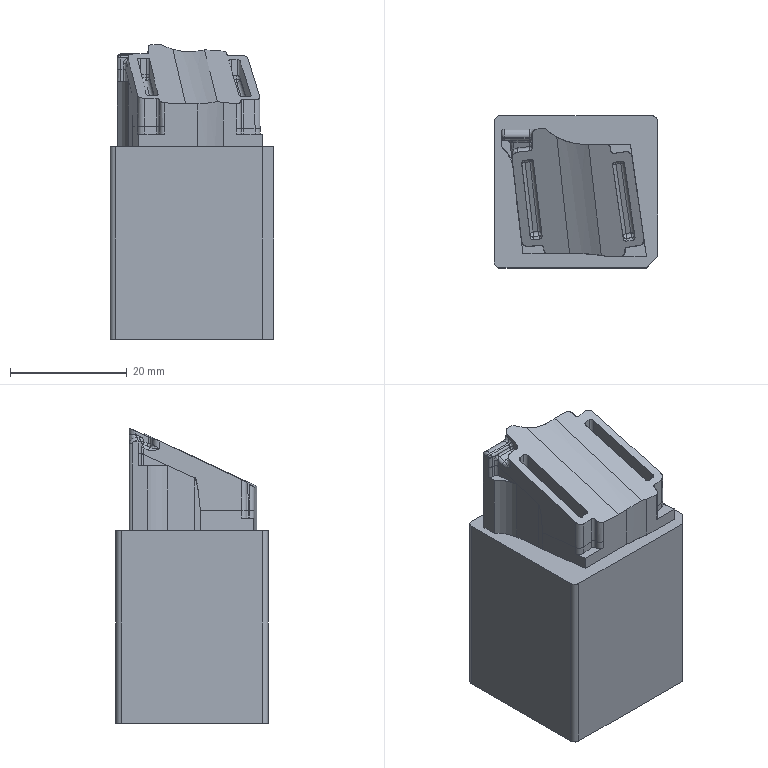NC program | NX | posted with a generic post | part box 28 x 26 x 50.455 mm
Whole program:
N10 G17 G21 G94 G90
(CONTOUR_AREA_1 , TOOL : D0.8R0.4)
N12 T00 M6
N14 G54
N16 G17 G0 G90 X-13.442 Y10.172 S0 M3
N18 G43 Z10. H0
N20 Z1.2
N22 G94 G1 Z-3.351 F250.
N24 X-13.296 Y10.317 Z-3.332
N26 X-13.177 Y10.437 Z-3.212
N28 X-13.116 Y10.498 Z-3.024
N30 X-13.077 Y10.536 Z-2.705
N32 X-13.039 Y10.575 Z-2.609
N34 X-12.962 Y10.652 Z-2.512
N36 X-12.931 Y10.683 Z-2.49
N38 X-12.761 Y10.853 Z-2.513
N40 X-12.628 Y10.986 Z-2.654
N42 X-12.591 Y11.022 Z-2.731
N44 X-12.553 Y11.061 Z-3.024
N46 X-12.381 Y11.093
N48 X-12.456 Y11.018 Z-2.583
N50 X-12.522 Y10.952 Z-2.469
N52 X-12.691 Y10.783 Z-2.308
N54 X-12.861 Y10.613 Z-2.274
N56 X-13.031 Y10.443 Z-2.381
N58 X-13.078 Y10.396 Z-2.465
N60 X-13.15 Y10.324 Z-3.024
N62 X-13.162 Y10.249
N64 X-13.163 Y10.171 Z-2.858
N66 X-13.13 Y10.204 Z-2.474
N68 X-13.102 Y10.232 Z-2.38
N70 X-12.961 Y10.373 Z-2.19
N72 X-12.791 Y10.543 Z-2.121
N74 X-12.621 Y10.713 Z-2.15
N76 X-12.452 Y10.882 Z-2.293
N78 X-12.368 Y10.966 Z-2.418
N80 X-12.282 Y11.052 Z-2.614
N82 X-12.249 Y11.085 Z-2.731
N84 X-12.217 Y11.118 Z-3.024
N86 X-12.077
N88 X-12.107 Y11.088 Z-2.745
N90 X-12.137 Y11.058 Z-2.627
N92 X-12.212 Y10.982 Z-2.437
N94 X-12.382 Y10.813 Z-2.179
N96 X-12.551 Y10.643 Z-2.046
N98 X-12.721 Y10.473 Z-2.005
N100 X-12.891 Y10.303 Z-2.04
N102 X-13.061 Y10.134 Z-2.215
N104 X-13.104 Y10.09 Z-2.295
N106 X-13.164 Y10.03 Z-2.61
N108 Y9.952 Z-2.586
N110 Y9.89 Z-2.531
N112 X-13.104 Y9.95 Z-2.236
N114 X-12.991 Y10.064 Z-2.055
N116 X-12.821 Y10.234 Z-1.943
N118 X-12.651 Y10.403 Z-1.907
N120 X-12.482 Y10.573 Z-1.961
N122 X-12.312 Y10.743 Z-2.075
N124 X-12.142 Y10.912 Z-2.3
N126 X-11.997 Y11.058 Z-2.627
N128 X-11.972 Y11.082 Z-2.716
N130 X-11.937 Y11.118 Z-3.024
N132 X-11.797
N134 X-11.827 Y11.088 Z-2.745
N136 X-11.857 Y11.058 Z-2.627
N138 X-11.903 Y11.012 Z-2.512
N140 X-12.072 Y10.842 Z-2.204
N142 X-12.242 Y10.673 Z-2.008
N144 X-12.412 Y10.503 Z-1.884
N146 X-12.581 Y10.333 Z-1.839
N148 X-12.751 Y10.164 Z-1.853
N150 X-12.921 Y9.994 Z-1.948
N152 X-13.09 Y9.824 Z-2.177
N154 X-13.104 Y9.811 Z-2.209
N156 X-13.164 Y9.751 Z-2.503
N158 Y9.611 Z-2.515
N160 X-13.104 Y9.671 Z-2.207
N162 X-13.021 Y9.754 Z-2.038
N164 X-12.851 Y9.924 Z-1.869
N166 X-12.681 Y10.094 Z-1.786
N168 X-12.511 Y10.263 Z-1.783
N170 X-12.342 Y10.433 Z-1.829
N172 X-12.172 Y10.603 Z-1.95
N174 X-12.002 Y10.773 Z-2.108
N176 X-11.833 Y10.942 Z-2.346
N178 X-11.717 Y11.058 Z-2.627
N180 X-11.687 Y11.088 Z-2.745
N182 X-11.657 Y11.118 Z-3.024
N184 X-11.518
N186 X-11.548 Y11.088 Z-2.745
N188 X-11.578 Y11.058 Z-2.627
N190 X-11.593 Y11.042 Z-2.588
N192 X-11.678 Y10.957 Z-2.375
N194 X-11.763 Y10.872 Z-2.245
N196 X-11.932 Y10.703 Z-2.032
N198 X-12.102 Y10.533 Z-1.892
N200 X-12.272 Y10.363 Z-1.79
N202 X-12.442 Y10.194 Z-1.729
N204 X-12.611 Y10.024 Z-1.736
N206 X-12.781 Y9.854 Z-1.798
N208 X-12.951 Y9.684 Z-1.952
N210 X-13.104 Y9.531 Z-2.225
N212 X-13.12 Y9.515 Z-2.284
N214 X-13.142 Y9.493 Z-2.369
N216 X-13.154 Y9.482 Z-2.439
N218 X-13.165 Y9.471 Z-2.572
N220 Y9.356 Z-2.641
N222 X-13.164 Y9.332 Z-2.62
N224 X-13.105 Y9.391 Z-2.272
N226 X-13.051 Y9.445 Z-2.137
N228 X-12.881 Y9.615 Z-1.88
N230 X-12.711 Y9.784 Z-1.747
N232 X-12.541 Y9.954 Z-1.699
N234 X-12.372 Y10.124 Z-1.694
N236 X-12.202 Y10.293 Z-1.757
N238 X-12.032 Y10.463 Z-1.839
N240 X-11.863 Y10.633 Z-1.975
N242 X-11.693 Y10.803 Z-2.149
N244 X-11.523 Y10.972 Z-2.411
N246 X-11.438 Y11.058 Z-2.627
N248 X-11.408 Y11.088 Z-2.745
N250 X-11.378 Y11.118 Z-3.024
N252 X-11.238
N254 X-11.261 Y11.095 Z-2.783
N256 X-11.284 Y11.072 Z-2.67
N258 X-11.298 Y11.058 Z-2.627
N260 X-11.453 Y10.902 Z-2.286
N262 X-11.623 Y10.733 Z-2.06
N264 X-11.793 Y10.563 Z-1.917
N266 X-11.962 Y10.393 Z-1.804
N268 X-12.132 Y10.223 Z-1.724
N270 X-12.302 Y10.054 Z-1.673
N272 X-12.471 Y9.884 Z-1.664
N274 X-12.641 Y9.714 Z-1.71
N276 X-12.811 Y9.545 Z-1.827
N278 X-12.981 Y9.375 Z-2.046
N280 X-13.04 Y9.315 Z-2.16
N282 X-13.1 Y9.256 Z-2.319
N284 X-13.157 Y9.198 Z-2.68
N286 X-13.152 Y9.092 Z-2.706
N288 X-13.15 Y9.066 Z-2.687
N290 X-13.094 Y9.122 Z-2.364
N292 X-13.08 Y9.135 Z-2.327
N294 X-13.002 Y9.214 Z-2.156
N296 X-12.996 Y9.22 Z-2.139
N298 X-12.911 Y9.305 Z-1.981
N300 X-12.741 Y9.475 Z-1.785
N302 X-12.571 Y9.644 Z-1.681
N304 X-12.402 Y9.814 Z-1.639
N306 X-12.232 Y9.984 Z-1.658
N308 X-12.062 Y10.154 Z-1.694
N310 X-11.892 Y10.323 Z-1.771
N312 X-11.723 Y10.493 Z-1.86
N314 X-11.553 Y10.663 Z-1.999
N316 X-11.383 Y10.832 Z-2.19
N318 X-11.214 Y11.002 Z-2.487
N320 X-11.158 Y11.058 Z-2.627
N322 X-11.128 Y11.088 Z-2.745
N324 X-11.098 Y11.118 Z-3.024
N326 X-10.958
N328 X-10.988 Y11.088 Z-2.745
N330 X-11.018 Y11.058 Z-2.627
N332 X-11.144 Y10.932 Z-2.329
N334 X-11.313 Y10.763 Z-2.094
N336 X-11.483 Y10.593 Z-1.941
N338 X-11.653 Y10.423 Z-1.818
N340 X-11.823 Y10.253 Z-1.738
N342 X-11.992 Y10.084 Z-1.677
N344 X-12.162 Y9.914 Z-1.644
N346 X-12.332 Y9.744 Z-1.631
N348 X-12.501 Y9.575 Z-1.669
N350 X-12.671 Y9.405 Z-1.766
N352 X-12.841 Y9.235 Z-1.939
N354 X-12.926 Y9.15 Z-2.065
N356 X-12.991 Y9.085 Z-2.199
N358 X-13.011 Y9.065 Z-2.232
N360 X-13.066 Y9.01 Z-2.367
N362 X-13.112 Y8.964 Z-2.705
N364 X-13.073 Y8.863
N366 X-13.027 Y8.91 Z-2.344
N368 X-12.941 Y8.996 Z-2.158
N370 X-12.843 Y9.093 Z-2.009
N372 X-12.8 Y9.136 Z-1.957
N374 X-12.771 Y9.165 Z-1.91
N376 X-12.601 Y9.335 Z-1.753
N378 X-12.432 Y9.505 Z-1.658
N380 X-12.262 Y9.674 Z-1.626
N382 X-12.092 Y9.844 Z-1.631
N384 X-11.922 Y10.014 Z-1.664
N386 X-11.753 Y10.184 Z-1.705
N388 X-11.583 Y10.353 Z-1.785
N390 X-11.413 Y10.523 Z-1.884
N392 X-11.244 Y10.693 Z-2.024
N394 X-11.074 Y10.862 Z-2.231
N396 X-10.904 Y11.032 Z-2.562
N398 X-10.879 Y11.058 Z-2.627
N400 X-10.849 Y11.088 Z-2.745
N402 X-10.819 Y11.118 Z-3.024
N404 X-10.679
N406 X-10.709 Y11.088 Z-2.745
N408 X-10.739 Y11.058 Z-2.627
N410 X-10.834 Y10.962 Z-2.386
N412 X-11.004 Y10.792 Z-2.135
N414 X-11.174 Y10.623 Z-1.966
N416 X-11.343 Y10.453 Z-1.833
N418 X-11.513 Y10.283 Z-1.752
N420 X-11.683 Y10.114 Z-1.683
N422 X-11.853 Y9.944 Z-1.65
N424 X-12.022 Y9.774 Z-1.626
N426 X-12.192 Y9.605 Z-1.629
N428 X-12.362 Y9.435 Z-1.661
N430 X-12.531 Y9.265 Z-1.752
N432 X-12.701 Y9.095 Z-1.903
N434 X-12.871 Y8.926 Z-2.11
N436 X-12.987 Y8.809 Z-2.375
N438 X-13.011 Y8.786 Z-2.464
N440 X-13.034 Y8.763 Z-2.665
N442 X-13.033 Y8.761 Z-2.704
N444 X-12.976 Y8.681 Z-2.668
N446 X-12.955 Y8.702 Z-2.478
N448 X-12.933 Y8.724 Z-2.375
N450 X-12.801 Y8.856 Z-2.085
N452 X-12.631 Y9.025 Z-1.889
N454 X-12.461 Y9.195 Z-1.753
N456 X-12.292 Y9.365 Z-1.676
N458 X-12.122 Y9.535 Z-1.638
N460 X-11.952 Y9.704 Z-1.626
N462 X-11.783 Y9.874 Z-1.637
N464 X-11.613 Y10.044 Z-1.669
N466 X-11.443 Y10.213 Z-1.719
N468 X-11.273 Y10.383 Z-1.799
N470 X-11.104 Y10.553 Z-1.908
N472 X-10.934 Y10.723 Z-2.05
N474 X-10.764 Y10.892 Z-2.273
N476 X-10.595 Y11.062 Z-2.638
N478 X-10.567 Y11.09 Z-2.757
N480 X-10.539 Y11.118 Z-3.024
N482 X-10.399
N484 X-10.429 Y11.088 Z-2.745
N486 X-10.459 Y11.058 Z-2.627
N488 X-10.525 Y10.992 Z-2.461
N490 X-10.694 Y10.822 Z-2.176
N492 X-10.864 Y10.653 Z-1.991
N494 X-11.034 Y10.483 Z-1.852
N496 X-11.204 Y10.313 Z-1.766
N498 X-11.373 Y10.144 Z-1.691
N500 X-11.543 Y9.974 Z-1.656
N502 X-11.713 Y9.804 Z-1.627
N504 X-11.882 Y9.634
N506 X-12.052 Y9.465 Z-1.647
N508 X-12.222 Y9.295 Z-1.698
N510 X-12.392 Y9.125 Z-1.767
N512 X-12.561 Y8.956 Z-1.893
N514 X-12.731 Y8.786 Z-2.073
N516 X-12.868 Y8.648 Z-2.376
N518 X-12.911 Y8.606 Z-2.703
N520 X-12.862 Y8.553
N522 X-12.84 Y8.537 Z-2.659
N524 X-12.819 Y8.558 Z-2.477
N526 X-12.797 Y8.58 Z-2.387
N528 X-12.661 Y8.716 Z-2.081
N530 X-12.491 Y8.886 Z-1.909
N532 X-12.322 Y9.055 Z-1.793
N534 X-12.152 Y9.225 Z-1.72
N536 X-11.982 Y9.395 Z-1.665
N538 X-11.813 Y9.565 Z-1.634
N540 X-11.643 Y9.734 Z-1.626
N542 X-11.473 Y9.904 Z-1.642
N544 X-11.303 Y10.074 Z-1.675
N546 X-11.134 Y10.243 Z-1.733
N548 X-10.964 Y10.413 Z-1.813
N550 X-10.794 Y10.583 Z-1.933
N552 X-10.625 Y10.752 Z-2.082
N554 X-10.455 Y10.922 Z-2.314
N556 X-10.319 Y11.058 Z-2.627
N558 X-10.285 Y11.092 Z-2.767
N560 X-10.259 Y11.118 Z-3.024
N562 X-10.12
N564 X-10.15 Y11.088 Z-2.745
N566 X-10.18 Y11.058 Z-2.627
N568 X-10.215 Y11.022 Z-2.537
N570 X-10.385 Y10.852 Z-2.218
N572 X-10.555 Y10.683 Z-2.016
N574 X-10.724 Y10.513 Z-1.875
N576 X-10.894 Y10.343 Z-1.78
N578 X-11.064 Y10.173 Z-1.701
N580 X-11.234 Y10.004 Z-1.662
N582 X-11.403 Y9.834 Z-1.63
N584 X-11.573 Y9.664 Z-1.626
N586 X-11.743 Y9.495 Z-1.643
N588 X-11.912 Y9.325 Z-1.688
N590 X-12.082 Y9.155 Z-1.743
N592 X-12.124 Y9.113 Z-1.762
N594 X-12.262 Y8.975 Z-1.826
N596 X-12.379 Y8.858 Z-1.897
N598 X-12.421 Y8.816 Z-1.929
N600 X-12.591 Y8.646 Z-2.099
N602 X-12.717 Y8.521 Z-2.391
N604 X-12.738 Y8.499 Z-2.468
N606 X-12.76 Y8.478 Z-2.67
N608 X-12.74 Y8.463 Z-2.703
N610 X-12.669 Y8.429
N612 X-12.624 Y8.474 Z-2.378
N614 X-12.521 Y8.576 Z-2.143
N616 X-12.352 Y8.746 Z-1.953
N618 X-12.245 Y8.852 Z-1.884
N620 X-11.98 Y9.117 Z-1.76
N622 X-11.842 Y9.255 Z-1.711
N624 X-11.673 Y9.425 Z-1.656
N626 X-11.503 Y9.594 Z-1.631
N628 X-11.333 Y9.764 Z-1.626
N630 X-11.164 Y9.934 Z-1.648
N632 X-10.994 Y10.104 Z-1.681
N634 X-10.824 Y10.273 Z-1.747
N636 X-10.655 Y10.443 Z-1.828
N638 X-10.485 Y10.613 Z-1.958
N640 X-10.315 Y10.782 Z-2.121
N642 X-10.145 Y10.952 Z-2.364
N644 X-10.04 Y11.058 Z-2.627
N646 X-10.01 Y11.088 Z-2.745
N648 X-9.98 Y11.118 Z-3.024
N650 X-9.84
N652 X-9.87 Y11.088 Z-2.745
N654 X-9.906 Y11.052 Z-2.613
N656 X-9.991 Y10.967 Z-2.398
N658 X-10.075 Y10.882 Z-2.259
N660 X-10.245 Y10.712 Z-2.041
N662 X-10.415 Y10.543 Z-1.9
N664 X-10.585 Y10.373 Z-1.794
N666 X-10.754 Y10.203 Z-1.714
N668 X-10.924 Y10.034 Z-1.667
N670 X-11.094 Y9.864 Z-1.635
N672 X-11.263 Y9.694 Z-1.626
N674 X-11.433 Y9.525 Z-1.639
N676 X-11.603 Y9.355 Z-1.678
N678 X-11.773 Y9.185 Z-1.733
N680 X-11.836 Y9.121 Z-1.757
N682 X-12.101 Y8.856 Z-1.882
N684 X-12.112 Y8.846 Z-1.887
N686 X-12.196 Y8.761 Z-1.94
N688 X-12.282 Y8.676 Z-1.992
N690 X-12.451 Y8.506 Z-2.2
N692 X-12.528 Y8.43 Z-2.393
N694 X-12.574 Y8.383 Z-2.659
N696 X-12.555 Y8.374 Z-2.703
N698 X-12.461 Y8.357 Z-2.907
N700 X-12.409 Y8.409 Z-2.369
N702 X-12.381 Y8.436 Z-2.301
N704 X-12.212 Y8.606 Z-2.054
N706 X-12.042 Y8.776 Z-1.929
N708 X-11.968 Y8.85 Z-1.885
N710 X-11.703 Y9.115 Z-1.76
N712 X-11.533 Y9.285 Z-1.701
N714 X-11.363 Y9.455 Z-1.649
N716 X-11.194 Y9.624 Z-1.627
N718 X-11.024 Y9.794 Z-1.626
N720 X-10.854 Y9.964 Z-1.654
N722 X-10.684 Y10.133 Z-1.688
N724 X-10.515 Y10.303 Z-1.761
N726 X-10.345 Y10.473 Z-1.845
N728 X-10.175 Y10.643 Z-1.983
N730 X-10.006 Y10.812 Z-2.162
N732 X-9.836 Y10.982 Z-2.436
N734 X-9.76 Y11.058 Z-2.627
N736 X-9.73 Y11.088 Z-2.745
N738 X-9.7 Y11.118 Z-3.024
N740 X-9.56
N742 X-9.596 Y11.082 Z-2.715
N744 X-9.62 Y11.058 Z-2.627
N746 X-9.766 Y10.912 Z-2.3
N748 X-9.936 Y10.742 Z-2.07
N750 X-10.105 Y10.573 Z-1.925
N752 X-10.275 Y10.403 Z-1.808
N754 X-10.445 Y10.233 Z-1.728
N756 X-10.615 Y10.064 Z-1.673
N758 X-10.784 Y9.894 Z-1.641
N760 X-10.954 Y9.724 Z-1.626
N762 X-11.124 Y9.554 Z-1.636
N764 X-11.293 Y9.385 Z-1.669
N766 X-11.463 Y9.215 Z-1.724
N768 X-11.548 Y9.13 Z-1.753
N770 X-11.559 Y9.12 Z-1.758
N772 X-11.824 Y8.854 Z-1.883
N774 X-11.887 Y8.791 Z-1.918
N776 X-11.972 Y8.706 Z-1.98
N778 X-12.142 Y8.536 Z-2.129
N780 X-12.291 Y8.387 Z-2.381
N782 X-12.312 Y8.367 Z-2.447
N784 X-12.342 Y8.336 Z-3.163
N786 X-12.274 Y8.323 Z-3.311
N788 X-12.247 Y8.322 Z-3.667
N790 X-12.216 Z-3.744
N792 X-12.202 Y8.337 Z-2.571
N794 X-12.187 Y8.352 Z-2.499
N796 X-12.157 Y8.381 Z-2.395
N798 X-12.072 Y8.466 Z-2.222
N800 X-11.902 Y8.636 Z-2.03
N802 X-11.733 Y8.806 Z-1.908
N804 X-11.69 Y8.848 Z-1.886
N806 X-11.425 Y9.113 Z-1.761
N808 X-11.414 Y9.124 Z-1.756
N810 X-11.393 Y9.145 Z-1.747
N812 X-11.223 Y9.315 Z-1.691
N814 X-11.054 Y9.485 Z-1.644
N816 X-10.884 Y9.654 Z-1.626
N818 X-10.714 Y9.824 Z-1.629
N820 X-10.545 Y9.994 Z-1.66
N822 X-10.375 Y10.163 Z-1.697
N824 X-10.205 Y10.333 Z-1.775
N826 X-10.036 Y10.503 Z-1.867
N828 X-9.866 Y10.673 Z-2.007
N830 X-9.696 Y10.842 Z-2.204
N832 X-9.526 Y11.012 Z-2.512
N834 X-9.481 Y11.058 Z-2.627
N836 X-9.451 Y11.088 Z-2.745
N838 X-9.421 Y11.118 Z-3.024
N840 X-9.281
N842 X-9.311 Y11.088 Z-2.745
N844 X-9.341 Y11.058 Z-2.627
N846 X-9.456 Y10.942 Z-2.345
N848 X-9.626 Y10.772 Z-2.107
N850 X-9.796 Y10.603 Z-1.95
N852 X-9.966 Y10.433 Z-1.822
N854 X-10.135 Y10.263 Z-1.742
N856 X-10.305 Y10.093 Z-1.679
N858 X-10.475 Y9.924 Z-1.646
N860 X-10.644 Y9.754 Z-1.626
N862 X-10.814 Y9.584 Z-1.632
N864 X-10.984 Y9.415 Z-1.659
N866 X-11.154 Y9.245 Z-1.714
N868 X-11.281 Y9.118 Z-1.759
N870 X-11.546 Y8.853 Z-1.884
N872 X-11.557 Y8.842 Z-1.889
N874 X-11.578 Y8.821 Z-1.9
N876 X-11.663 Y8.736 Z-1.958
N878 X-11.832 Y8.566 Z-2.092
N880 X-12.002 Y8.396 Z-2.357
N882 X-12.018 Y8.38 Z-2.399
N884 X-12.048 Y8.35 Z-2.507
N886 X-12.063 Y8.336 Z-2.582
N888 X-12.078 Y8.321 Z-4.086
N890 X-11.939 Y8.319 Z-4.631
N892 X-11.924 Y8.334 Z-2.592
N894 X-11.909 Y8.349 Z-2.515
N896 X-11.879 Y8.379 Z-2.402
N898 X-11.762 Y8.496 Z-2.181
N900 X-11.593 Y8.666 Z-2.008
N902 X-11.423 Y8.836 Z-1.892
N904 X-11.412 Y8.846 Z-1.887
N906 X-11.402 Y8.857 Z-1.882
N908 X-11.137 Y9.122 Z-1.757
N910 X-11.126 Y9.133 Z-1.752
N912 X-11.084 Y9.175 Z-1.737
N914 X-10.914 Y9.345 Z-1.682
N916 X-10.744 Y9.514 Z-1.641
N918 X-10.575 Y9.684 Z-1.626
N920 X-10.405 Y9.854 Z-1.633
N922 X-10.235 Y10.024 Z-1.665
N924 X-10.065 Y10.193 Z-1.709
N926 X-9.896 Y10.363 Z-1.789
N928 X-9.726 Y10.533 Z-1.892
N930 X-9.556 Y10.702 Z-2.032
N932 X-9.387 Y10.872 Z-2.245
N934 X-9.302 Y10.957 Z-2.375
N936 X-9.217 Y11.042 Z-2.587
N938 X-9.201 Y11.058 Z-2.627
N940 X-9.171 Y11.088 Z-2.745
N942 X-9.141 Y11.118 Z-3.024
N944 X-9.001
N946 X-9.031 Y11.088 Z-2.745
N948 X-9.061 Y11.058 Z-2.627
N950 X-9.147 Y10.972 Z-2.411
N952 X-9.317 Y10.802 Z-2.149
N954 X-9.486 Y10.633 Z-1.974
N956 X-9.656 Y10.463 Z-1.839
N958 X-9.826 Y10.293 Z-1.756
N960 X-9.996 Y10.123 Z-1.685
N962 X-10.165 Y9.954 Z-1.652
N964 X-10.335 Y9.784 Z-1.626
N966 X-10.505 Y9.614 Z-1.628
N968 X-10.674 Y9.445 Z-1.651
N970 X-10.844 Y9.275 Z-1.704
N972 X-11.003 Y9.116 Z-1.76
N974 X-11.268 Y8.851 Z-1.885
N976 X-11.353 Y8.766 Z-1.935
N978 X-11.523 Y8.596 Z-2.062
N980 X-11.693 Y8.426 Z-2.297
N982 X-11.741 Y8.378 Z-2.404
N984 X-11.785 Y8.334 Z-2.597
N986 X-11.8 Y8.319 Z-3.985
N988 X-11.747
N990 X-11.686 Y8.294 Z-3.7
N992 Y8.293 Z-3.702
N994 X-11.656 Y8.323 Z-3.195
N996 X-11.653 Y8.326 Z-2.68
N998 X-11.643 Y8.336 Z-2.582
N1000 X-11.623 Y8.356 Z-2.499
N1002 X-11.538 Y8.441 Z-2.267
N1004 X-11.453 Y8.526 Z-2.142
N1006 X-11.283 Y8.696 Z-1.986
N1008 X-11.198 Y8.781 Z-1.924
N1010 X-11.156 Y8.823 Z-1.898
N1012 X-11.135 Y8.844 Z-1.888
N1014 X-11.124 Y8.855 Z-1.883
N1016 X-10.859 Y9.12 Z-1.758
N1018 X-10.774 Y9.205 Z-1.727
N1020 X-10.604 Y9.375 Z-1.672
N1022 X-10.435 Y9.544 Z-1.637
N1024 X-10.265 Y9.714 Z-1.626
N1026 X-10.095 Y9.884 Z-1.639
N1028 X-9.926 Y10.054 Z-1.671
N1030 X-9.756 Y10.223 Z-1.724
N1032 X-9.586 Y10.393 Z-1.803
N1034 X-9.417 Y10.563 Z-1.916
N1036 X-9.247 Y10.732 Z-2.06
N1038 X-9.077 Y10.902 Z-2.286
N1040 X-8.922 Y11.058 Z-2.627
N1042 X-8.907 Y11.072 Z-2.669
N1044 X-8.884 Y11.095 Z-2.782
N1046 X-8.862 Y11.118 Z-3.024
N1048 X-8.722
N1050 X-8.752 Y11.088 Z-2.745
N1052 X-8.782 Y11.058 Z-2.627
N1054 X-8.838 Y11.002 Z-2.486
N1056 X-9.007 Y10.832 Z-2.19
N1058 X-9.177 Y10.662 Z-1.999
N1060 X-9.347 Y10.493 Z-1.859
N1062 X-9.516 Y10.323 Z-1.771
N1064 X-9.686 Y10.153 Z-1.694
N1066 X-9.856 Y9.984 Z-1.658
N1068 X-10.025 Y9.814 Z-1.628
N1070 X-10.195 Y9.644 Z-1.626
N1072 X-10.365 Y9.474 Z-1.646
N1074 X-10.535 Y9.305 Z-1.695
N1076 X-10.704 Y9.135 Z-1.751
N1078 X-10.715 Y9.124 Z-1.756
N1080 X-10.725 Y9.114 Z-1.761
N1082 X-10.991 Y8.849 Z-1.886
N1084 X-11.001 Y8.838 Z-1.891
N1086 X-11.044 Y8.796 Z-1.914
N1088 X-11.213 Y8.626 Z-2.037
N1090 X-11.383 Y8.456 Z-2.239
N1092 X-11.468 Y8.371 Z-2.428
N1094 X-11.51 Y8.329 Z-2.651
N1096 X-11.521 Y8.318 Z-3.042
N1098 X-11.532 Y8.308 Z-3.117
N1100 X-11.553 Y8.287 Z-3.237
N1102 X-11.594 Y8.245 Z-3.372
N1104 X-11.62 Y8.219 Z-3.489
N1106 X-11.646 Y8.193 Z-3.724
N1108 X-11.632 Y8.068 Z-3.787
N1110 X-11.577 Y8.122 Z-3.422
N1112 X-11.483 Y8.217 Z-3.169
N1114 X-11.429 Y8.271 Z-3.051
N1116 X-11.402 Y8.298 Z-2.993
N1118 X-11.375 Y8.325 Z-2.844
N1120 X-11.359 Y8.34 Z-2.564
N1122 X-11.344 Y8.356 Z-2.503
N1124 X-11.313 Y8.386 Z-2.382
N1126 X-11.143 Y8.556 Z-2.105
N1128 X-10.974 Y8.726 Z-1.964
N1130 X-10.857 Y8.842 Z-1.889
N1132 X-10.847 Y8.853 Z-1.884
N1134 X-10.581 Y9.118 Z-1.759
N1136 X-10.465 Y9.235 Z-1.717
N1138 X-10.295 Y9.405 Z-1.662
N1140 X-10.125 Y9.574 Z-1.633
N1142 X-9.956 Y9.744 Z-1.626
N1144 X-9.786 Y9.914 Z-1.644
N1146 X-9.616 Y10.083 Z-1.677
N1148 X-9.446 Y10.253 Z-1.738
N1150 X-9.277 Y10.423 Z-1.818
N1152 X-9.107 Y10.593 Z-1.941
N1154 X-8.937 Y10.762 Z-2.094
N1156 X-8.768 Y10.932 Z-2.329
N1158 X-8.642 Y11.058 Z-2.627
N1160 X-8.612 Y11.088 Z-2.745
N1162 X-8.582 Y11.118 Z-3.024
N1164 X-8.442
N1166 X-8.472 Y11.088 Z-2.745
N1168 X-8.502 Y11.058 Z-2.627
N1170 X-8.528 Y11.032 Z-2.562
N1172 X-8.698 Y10.862 Z-2.231
N1174 X-8.867 Y10.692 Z-2.024
N1176 X-9.037 Y10.523 Z-1.883
N1178 X-9.207 Y10.353 Z-1.785
N1180 X-9.377 Y10.183 Z-1.705
N1182 X-9.546 Y10.014 Z-1.663
N1184 X-9.716 Y9.844 Z-1.631
N1186 X-9.886 Y9.674 Z-1.626
N1188 X-10.055 Y9.504 Z-1.642
N1190 X-10.225 Y9.335 Z-1.685
N1192 X-10.395 Y9.165 Z-1.74
N1194 X-10.437 Y9.123 Z-1.757
N1196 X-10.448 Y9.112 Z-1.762
N1198 X-10.702 Y8.857 Z-1.881
N1200 X-10.713 Y8.847 Z-1.886
N1202 X-10.734 Y8.826 Z-1.897
N1204 X-10.904 Y8.656 Z-2.015
N1206 X-11.074 Y8.486 Z-2.194
N1208 X-11.158 Y8.401 Z-2.348
N1210 X-11.201 Y8.359 Z-2.486
N1212 X-11.222 Y8.338 Z-2.579
N1214 X-11.234 Y8.326 Z-2.705
N1216 X-11.243 Y8.316 Z-2.826
N1218 X-11.286 Y8.274 Z-2.917
N1220 X-11.328 Y8.232 Z-2.983
N1222 X-11.413 Y8.147 Z-3.12
N1224 X-11.563 Y7.997 Z-3.48
N1226 X-11.583 Y7.977 Z-3.572
N1228 X-11.617 Y7.943 Z-3.832
N1230 X-11.602 Y7.818 Z-3.886
N1232 X-11.548 Y7.872 Z-3.536
N1234 X-11.513 Y7.907 Z-3.433
N1236 X-11.343 Y8.077 Z-3.085
N1238 X-11.173 Y8.247 Z-2.866
N1240 X-11.131 Y8.289 Z-2.816
N1242 X-11.11 Y8.31 Z-2.783
N1244 X-11.105 Y8.315 Z-2.77
N1246 X-11.099 Y8.321 Z-2.75
N1248 Z-2.748
N1250 X-11.094 Y8.326 Z-2.699
N1252 X-11.089 Y8.331 Z-2.617
N1254 X-11.004 Y8.416 Z-2.316
N1256 X-10.834 Y8.586 Z-2.072
N1258 X-10.664 Y8.756 Z-1.941
N1260 X-10.579 Y8.841 Z-1.889
N1262 X-10.569 Y8.851 Z-1.884
N1264 X-10.304 Y9.116 Z-1.76
N1266 X-10.155 Y9.265 Z-1.708
N1268 X-9.985 Y9.435 Z-1.654
N1270 X-9.816 Y9.604 Z-1.629
N1272 X-9.646 Y9.774 Z-1.626
N1274 X-9.476 Y9.944 Z-1.65
N1276 X-9.307 Y10.113 Z-1.683
N1278 X-9.137 Y10.283 Z-1.752
N1280 X-8.967 Y10.453 Z-1.833
N1282 X-8.798 Y10.622 Z-1.966
N1284 X-8.628 Y10.792 Z-2.135
N1286 X-8.458 Y10.962 Z-2.386
N1288 X-8.362 Y11.058 Z-2.627
N1290 X-8.332 Y11.088 Z-2.745
N1292 X-8.302 Y11.118 Z-3.024
N1294 X-8.163
N1296 X-8.191 Y11.09 Z-2.756
N1298 X-8.219 Y11.062 Z-2.638
N1300 X-8.388 Y10.892 Z-2.272
N1302 X-8.558 Y10.722 Z-2.05
N1304 X-8.728 Y10.553 Z-1.908
N1306 X-8.897 Y10.383 Z-1.799
N1308 X-9.067 Y10.213 Z-1.719
N1310 X-9.237 Y10.043 Z-1.669
N1312 X-9.406 Y9.874 Z-1.637
N1314 X-9.576 Y9.704 Z-1.626
N1316 X-9.746 Y9.534 Z-1.638
N1318 X-9.916 Y9.365 Z-1.675
N1320 X-10.085 Y9.195 Z-1.73
N1322 X-10.16 Y9.121 Z-1.758
N1324 X-10.425 Y8.856 Z-1.882
N1326 X-10.51 Y8.771 Z-1.93
N1328 X-10.594 Y8.686 Z-1.993
N1330 X-10.764 Y8.516 Z-2.155
N1332 X-10.849 Y8.431 Z-2.287
N1334 X-10.934 Y8.346 Z-2.546
N1336 X-10.955 Y8.325 Z-2.668
N1338 X-10.977 Y8.304 Z-2.746
N1340 X-10.998 Y8.282 Z-2.773
N1342 X-11.041 Y8.239 Z-2.815
N1344 X-11.104 Y8.177 Z-2.869
N1346 X-11.273 Y8.007 Z-3.064
N1348 X-11.443 Y7.837 Z-3.348
N1350 X-11.534 Y7.747 Z-3.594
N1352 X-11.588 Y7.692 Z-3.945
N1354 X-11.573 Y7.567 Z-4.004
N1356 X-11.543 Y7.598 Z-3.763
N1358 X-11.519 Y7.621 Z-3.651
N1360 X-11.373 Y7.767 Z-3.299
N1362 X-11.203 Y7.937 Z-3.05
N1364 X-11.034 Y8.107 Z-2.879
N1366 X-10.949 Y8.192 Z-2.815
N1368 X-10.864 Y8.276 Z-2.754
N1370 X-10.821 Y8.319 Z-2.691
N1372 X-10.779 Y8.361 Z-2.471
N1374 X-10.694 Y8.446 Z-2.258
N1376 X-10.524 Y8.616 Z-2.044
N1378 X-10.355 Y8.786 Z-1.92
N1380 X-10.291 Y8.849 Z-1.885
N1382 X-10.026 Y9.114 Z-1.761
N1384 X-10.015 Y9.125 Z-1.756
N1386 X-9.846 Y9.295 Z-1.698
N1388 X-9.676 Y9.464 Z-1.647
N1390 X-9.506 Y9.634 Z-1.627
N1392 X-9.337 Y9.804
N1394 X-9.167 Y9.974 Z-1.656
N1396 X-8.997 Y10.143 Z-1.691
N1398 X-8.827 Y10.313 Z-1.766
N1400 X-8.658 Y10.483 Z-1.852
N1402 X-8.488 Y10.652 Z-1.991
N1404 X-8.318 Y10.822 Z-2.176
N1406 X-8.149 Y10.992 Z-2.461
N1408 X-8.083 Y11.058 Z-2.627
N1410 X-8.053 Y11.088 Z-2.745
N1412 X-8.023 Y11.118 Z-3.024
N1414 X-7.883 Z-3.007
N1416 X-7.909 Y11.092 Z-2.75
N1418 X-7.943 Y11.058 Z-2.637
N1420 X-8.011 Y10.99 Z-2.445
N1422 X-8.028 Y10.973 Z-2.405
N1424 X-8.079 Y10.922 Z-2.313
N1426 X-8.248 Y10.752 Z-2.082
N1428 X-8.418 Y10.582 Z-1.933
N1430 X-8.588 Y10.413 Z-1.813
N1432 X-8.758 Y10.243 Z-1.733
N1434 X-8.927 Y10.073 Z-1.675
N1436 X-9.097 Y9.904 Z-1.642
N1438 X-9.267 Y9.734 Z-1.626
N1440 X-9.436 Y9.564 Z-1.634
N1442 X-9.606 Y9.395 Z-1.666
N1444 X-9.776 Y9.225 Z-1.721
N1446 X-9.882 Y9.119 Z-1.759
N1448 X-10.147 Y8.854 Z-1.883
N1450 X-10.158 Y8.843 Z-1.888
N1452 X-10.2 Y8.801 Z-1.911
N1454 X-10.285 Y8.716 Z-1.971
N1456 X-10.455 Y8.546 Z-2.118
N1458 X-10.624 Y8.376 Z-2.41
N1460 X-10.675 Y8.326 Z-2.649
N1462 X-10.704 Y8.296 Z-2.731
N1464 X-10.764 Y8.236 Z-2.774
N1466 X-10.779 Y8.222 Z-2.781
N1468 X-10.794 Y8.207 Z-2.788
N1470 X-10.964 Y8.037 Z-2.891
N1472 X-11.133 Y7.867 Z-3.044
N1474 X-11.303 Y7.697 Z-3.263
N1476 X-11.473 Y7.528 Z-3.614
N1478 X-11.505 Y7.496 Z-3.709
N1480 X-11.559 Y7.442 Z-4.059
N1482 X-11.544 Y7.317 Z-4.109
N1484 X-11.53 Y7.33 Z-3.956
N1486 X-11.49 Y7.371 Z-3.766
N1488 X-11.403 Y7.458 Z-3.528
N1490 X-11.233 Y7.628 Z-3.24
N1492 X-11.064 Y7.797 Z-3.045
N1494 X-10.894 Y7.967 Z-2.913
N1496 X-10.756 Y8.105 Z-2.834
N1498 X-10.629 Y8.232 Z-2.776
N1500 X-10.618 Y8.243 Z-2.77
N1502 X-10.597 Y8.264 Z-2.757
N1504 X-10.554 Y8.306 Z-2.719
N1506 X-10.512 Y8.349 Z-2.531
N1508 X-10.47 Y8.391 Z-2.372
N1510 X-10.385 Y8.476 Z-2.208
N1512 X-10.215 Y8.646 Z-2.021
N1514 X-10.045 Y8.816 Z-1.902
N1516 X-10.003 Y8.858 Z-1.881
N1518 X-9.748 Y9.113 Z-1.762
N1520 X-9.706 Y9.155 Z-1.743
N1522 X-9.536 Y9.325 Z-1.688
N1524 X-9.366 Y9.494 Z-1.643
N1526 X-9.197 Y9.664 Z-1.626
N1528 X-9.027 Y9.834 Z-1.63
N1530 X-8.857 Y10.003 Z-1.662
N1532 X-8.688 Y10.173 Z-1.701
N1534 X-8.518 Y10.343 Z-1.78
N1536 X-8.348 Y10.513 Z-1.875
N1538 X-8.179 Y10.682 Z-2.016
N1540 X-8.009 Y10.852 Z-2.217
N1542 X-7.988 Y10.873 Z-2.247
N1544 X-7.924 Y10.937 Z-2.327
N1546 X-7.839 Y11.022 Z-2.513
N1548 X-7.803 Y11.058 Z-2.603
N1550 X-7.773 Y11.088 Z-2.717
N1552 X-7.743 Y11.118 Z-2.994
N1554 X-7.636 Z-2.968
N1556 X-7.603 Z-2.955
N1558 X-7.633 Y11.088 Z-2.67
N1560 X-7.663 Y11.058 Z-2.557
N1562 X-7.769 Y10.952 Z-2.315
N1564 X-7.939 Y10.782 Z-2.113
N1566 X-8.109 Y10.612 Z-1.958
N1568 X-8.278 Y10.443 Z-1.828
N1570 X-8.448 Y10.273 Z-1.747
N1572 X-8.618 Y10.103 Z-1.681
N1574 X-8.787 Y9.934 Z-1.648
N1576 X-8.957 Y9.764 Z-1.626
N1578 X-9.127 Y9.594 Z-1.631
N1580 X-9.297 Y9.424 Z-1.656
N1582 X-9.466 Y9.255 Z-1.711
N1584 X-9.604 Y9.117 Z-1.76
N1586 X-9.869 Y8.852 Z-1.884
N1588 X-9.975 Y8.746 Z-1.948
N1590 X-10.145 Y8.576 Z-2.082
N1592 X-10.315 Y8.406 Z-2.339
N1594 X-10.395 Y8.326 Z-2.649
N1596 X-10.417 Y8.304 Z-2.723
N1598 X-10.44 Y8.281 Z-2.746
N1600 X-10.485 Y8.237 Z-2.774
N1602 X-10.75 Y7.971 Z-2.895
N1604 X-10.824 Y7.897 Z-2.936
N1606 X-10.994 Y7.727 Z-3.055
N1608 X-11.163 Y7.558 Z-3.225
N1610 X-11.333 Y7.388 Z-3.478
N1612 X-11.404 Y7.317 Z-3.621
N1614 X-11.475 Y7.246 Z-3.817
N1616 X-11.503 Y7.218 Z-3.923
N1618 X-11.529 Y7.192 Z-4.149
N1620 X-11.515 Y7.067 Z-4.176
N1622 X-11.46 Y7.121 Z-3.848
N1624 X-11.433 Y7.148 Z-3.771
N1626 X-11.263 Y7.318 Z-3.441
N1628 X-11.093 Y7.488 Z-3.221
N1630 X-10.924 Y7.657 Z-3.066
N1632 X-10.754 Y7.827 Z-2.962
N1634 X-10.743 Y7.838 Z-2.956
N1636 X-10.733 Y7.848 Z-2.951
N1638 X-10.355 Y8.226 Z-2.778
N1640 X-10.335 Y8.246 Z-2.768
N1642 X-10.295 Y8.286 Z-2.742
N1644 X-10.255 Y8.326 Z-2.649
N1646 X-10.245 Y8.336 Z-2.592
N1648 X-10.16 Y8.421 Z-2.306
N1650 X-10.075 Y8.506 Z-2.169
N1652 X-9.905 Y8.676 Z-1.999
N1654 X-9.736 Y8.845 Z-1.887
N1656 X-9.725 Y8.856 Z-1.882
N1658 X-9.46 Y9.121 Z-1.758
N1660 X-9.396 Y9.185 Z-1.733
N1662 X-9.227 Y9.355 Z-1.678
N1664 X-9.057 Y9.524 Z-1.639
N1666 X-8.887 Y9.694 Z-1.626
N1668 X-8.718 Y9.864 Z-1.635
N1670 X-8.548 Y10.033 Z-1.667
N1672 X-8.378 Y10.203 Z-1.714
N1674 X-8.208 Y10.373 Z-1.794
N1676 X-8.039 Y10.542 Z-1.9
N1678 X-7.996 Y10.585 Z-1.93
N1680 X-7.954 Y10.627 Z-1.96
N1682 X-7.869 Y10.712 Z-2.01
N1684 X-7.699 Y10.882 Z-2.167
N1686 X-7.53 Y11.052 Z-2.478
N1688 X-7.494 Y11.088 Z-2.61
N1690 X-7.464 Y11.118 Z-2.905
N1692 X-7.324 Z-2.836
N1694 X-7.354 Y11.088 Z-2.522
N1696 X-7.384 Y11.058 Z-2.406
N1698 X-7.46 Y10.982 Z-2.201
N1700 X-7.629 Y10.812 Z-1.988
N1702 X-7.799 Y10.642 Z-1.906
N1704 X-7.969 Y10.473 Z-1.838
N1706 X-8.054 Y10.388 Z-1.798
N1708 X-8.139 Y10.303 Z-1.761
N1710 X-8.308 Y10.133 Z-1.688
N1712 X-8.478 Y9.963 Z-1.654
N1714 X-8.648 Y9.794 Z-1.626
N1716 X-8.817 Y9.624 Z-1.627
N1718 X-8.987 Y9.454 Z-1.649
N1720 X-9.157 Y9.285 Z-1.701
N1722 X-9.326 Y9.115 Z-1.761
N1724 X-9.592 Y8.85 Z-1.885
N1726 X-9.666 Y8.776 Z-1.926
N1728 X-9.836 Y8.606 Z-2.052
N1730 X-10.005 Y8.436 Z-2.277
N1732 X-10.09 Y8.351 Z-2.516
N1734 X-10.133 Y8.309 Z-2.714
N1736 X-10.175 Y8.266 Z-2.755
N1738 X-10.196 Y8.245 Z-2.769
N1740 X-10.207 Y8.235 Z-2.775
N1742 X-10.716 Y7.725 Z-3.008
N1744 X-10.854 Y7.588 Z-3.086
N1746 X-11.024 Y7.418 Z-3.22
N1748 X-11.193 Y7.248 Z-3.418
N1750 X-11.363 Y7.078 Z-3.682
N1752 X-11.446 Y6.996 Z-3.88
N1754 X-11.5 Y6.942 Z-4.195
N1756 X-11.485 Y6.817 Z-4.205
N1758 X-11.463 Y6.839 Z-4.034
N1760 X-11.431 Y6.871 Z-3.897
N1762 X-11.293 Y7.009 Z-3.626
N1764 X-11.208 Y7.093 Z-3.509
N1766 X-11.123 Y7.178 Z-3.402
N1768 X-10.954 Y7.348 Z-3.23
N1770 X-10.784 Y7.518 Z-3.11
N1772 X-10.699 Y7.603 Z-3.064
N1774 X-10.073 Y8.229 Z-2.777
N1776 X-10.008 Y8.294 Z-2.734
N1778 X-9.976 Y8.326 Z-2.649
N1780 X-9.935 Y8.366 Z-2.444
N1782 X-9.766 Y8.536 Z-2.131
N1784 X-9.596 Y8.706 Z-1.977
N1786 X-9.511 Y8.79 Z-1.916
N1788 X-9.448 Y8.854 Z-1.883
N1790 X-9.182 Y9.119 Z-1.758
N1792 X-9.172 Y9.13 Z-1.754
N1794 X-9.087 Y9.215 Z-1.724
N1796 X-8.917 Y9.384 Z-1.669
N1798 X-8.747 Y9.554 Z-1.636
N1800 X-8.578 Y9.724 Z-1.626
N1802 X-8.408 Y9.894 Z-1.64
N1804 X-8.238 Y10.063 Z-1.673
N1806 X-8.069 Y10.233 Z-1.728
N1808 X-7.984 Y10.318 Z-1.759
N1810 X-7.899 Y10.403 Z-1.766
N1812 X-7.729 Y10.572 Z-1.738
N1814 X-7.56 Y10.742 Z-1.752
N1816 X-7.475 Y10.827 Z-1.785
N1818 X-7.39 Y10.912 Z-1.93
N1820 X-7.317 Y10.985 Z-2.045
N1822 X-7.22 Y11.082 Z-2.36
N1824 X-7.202 Y11.1 Z-2.484
N1826 X-7.184 Y11.118 Z-2.732
N1828 X-7.044 Z-2.633
N1830 X-7.074 Y11.088 Z-2.242
N1832 X-7.104 Y11.058 Z-2.094
N1834 X-7.15 Y11.012 Z-1.896
N1836 X-7.217 Y10.945 Z-1.681
N1838 X-7.25 Y10.912 Z-1.538
N1840 X-7.267 Y10.895 Z-1.435
N1842 X-7.284 Y10.878 Z-1.366
N1844 X-6.996 Y11.026 Z-1.38
N1846 X-6.984 Y11.038 Z-1.631
N1848 X-6.95 Y11.072 Z-1.884
N1850 X-6.927 Y11.095 Z-2.132
N1852 X-6.904 Y11.118 Z-2.484
N1854 X-6.765 Z-2.27
N1856 X-6.781 Y11.101 Z-1.941
N1858 X-6.797 Y11.085 Z-1.408
N1860 X-6.631 Y11.111 Z-1.747
N1862 X-6.625 Y11.118 Z-2.003
N1864 X-6.582 Y11.161 Z-2.201
N1866 X-6.475 Y11.268 Z-2.342
N1868 X-6.332 Y11.41 Z-2.388
N1870 Z2.96
N1872 G0 Z10.
N1874 X-11.529 Y7.191
N1876 Z1.2
N1878 G1 Z-3.781
N1880 X-11.524 Y7.149 Z-3.983
N1882 X-11.508 Y7.012 Z-4.138
N1884 X-11.485 Y6.817 Z-4.202
N1886 X-11.47 Y6.692 Z-4.209
N1888 X-11.416 Y6.746 Z-3.889
N1890 X-11.393 Y6.769 Z-3.831
N1892 X-11.223 Y6.939 Z-3.572
N1894 X-11.053 Y7.108 Z-3.394
N1896 X-10.884 Y7.278 Z-3.242
N1898 X-10.714 Y7.448 Z-3.136
N1900 X-10.693 Y7.469 Z-3.125
N1902 X-10.682 Y7.48 Z-3.12
N1904 X-9.929 Y8.233 Z-2.776
N1906 X-9.866 Y8.296 Z-2.731
N1908 X-9.844 Y8.318 Z-2.695
N1910 X-9.823 Y8.339 Z-2.578
N1912 X-9.781 Y8.381 Z-2.397
N1914 X-9.696 Y8.466 Z-2.223
N1916 X-9.526 Y8.636 Z-2.028
N1918 X-9.356 Y8.805 Z-1.908
N1920 X-9.314 Y8.848 Z-1.886
N1922 X-9.049 Y9.113 Z-1.761
N1924 X-9.038 Y9.124 Z-1.756
N1926 X-9.017 Y9.145 Z-1.747
N1928 X-8.847 Y9.315 Z-1.691
N1930 X-8.678 Y9.484 Z-1.645
N1932 X-8.508 Y9.654 Z-1.626
N1934 X-8.338 Y9.824 Z-1.629
N1936 X-8.168 Y9.993 Z-1.66
N1938 X-7.999 Y10.163 Z-1.692
N1940 X-7.829 Y10.333 Z-1.621
N1942 X-7.736 Y10.426 Z-1.525
N1944 X-7.699 Y10.463 Z-1.453
N1946 X-7.68 Y10.482 Z-1.391
N1948 X-7.661 Y10.501 Z-1.362
N1950 X-7.798 Y10.249 Z-1.369
N1952 X-7.812 Y10.21 Z-1.37
N1954 X-7.837 Y10.186 Z-1.471
N1956 X-7.861 Y10.161 Z-1.53
N1958 X-7.909 Y10.113 Z-1.595
N1960 X-7.929 Y10.093 Z-1.614
N1962 X-8. Y10.022 Z-1.657
N1964 X-8.086 Y9.936 Z-1.649
N1966 X-8.099 Y9.924 Z-1.646
N1968 X-8.268 Y9.754 Z-1.626
N1970 X-8.438 Y9.584 Z-1.632
N1972 X-8.608 Y9.414 Z-1.659
N1974 X-8.777 Y9.245 Z-1.714
N1976 X-8.905 Y9.117 Z-1.759
N1978 X-9.17 Y8.852 Z-1.884
N1980 X-9.287 Y8.736 Z-1.954
N1982 X-9.456 Y8.566 Z-2.094
N1984 X-9.626 Y8.396 Z-2.363
N1986 X-9.696 Y8.326 Z-2.649
N1988 X-9.746 Y8.276 Z-2.749
N1990 X-9.771 Y8.251 Z-2.765
N1992 X-9.783 Y8.239 Z-2.773
N1994 X-10.676 Y7.346 Z-3.181
N1996 X-10.814 Y7.208 Z-3.259
N1998 X-10.984 Y7.039 Z-3.387
N2000 X-11.153 Y6.869 Z-3.522
N2002 X-11.323 Y6.699 Z-3.723
N2004 X-11.401 Y6.621 Z-3.88
N2006 X-11.455 Y6.567 Z-4.188
N2008 X-11.439 Y6.443 Z-4.159
N2010 X-11.386 Y6.497 Z-3.864
N2012 X-11.253 Y6.629 Z-3.63
N2014 X-11.083 Y6.799 Z-3.476
N2016 X-10.914 Y6.969 Z-3.374
N2018 X-10.829 Y7.053 Z-3.329
N2020 X-10.744 Y7.138 Z-3.284
N2022 X-10.659 Y7.223 Z-3.238
N2024 X-9.651 Y8.231 Z-2.776
N2026 X-9.641 Y8.241 Z-2.771
N2028 X-9.598 Y8.284 Z-2.744
N2030 X-9.556 Y8.326 Z-2.648
N2032 X-9.471 Y8.411 Z-2.33
N2034 X-9.386 Y8.496 Z-2.182
N2036 X-9.217 Y8.666 Z-2.006
N2038 X-9.047 Y8.835 Z-1.892
N2040 X-9.036 Y8.846 Z-1.887
N2042 X-9.026 Y8.857 Z-1.882
N2044 X-8.761 Y9.122 Z-1.757
N2046 X-8.75 Y9.132 Z-1.753
N2048 X-8.707 Y9.175 Z-1.737
N2050 X-8.538 Y9.344 Z-1.682
N2052 X-8.368 Y9.514 Z-1.641
N2054 X-8.198 Y9.684 Z-1.626
N2056 X-8.029 Y9.854 Z-1.633
N2058 X-7.987 Y9.895 Z-1.613
N2060 X-7.946 Y9.936 Z-1.575
N2062 X-7.909 Y9.974 Z-1.519
N2064 X-7.871 Y10.011 Z-1.362
N2066 X-7.885 Y9.952 Z-1.361
N2068 X-7.893 Y9.85 Z-1.373
N2070 X-7.925 Y9.817 Z-1.499
N2072 X-7.959 Y9.784 Z-1.568
N2074 X-8.012 Y9.73 Z-1.624
N2076 X-8.128 Y9.614 Z-1.628
N2078 X-8.298 Y9.444 Z-1.651
N2080 X-8.468 Y9.275 Z-1.704
N2082 X-8.627 Y9.115 Z-1.76
N2084 X-8.892 Y8.85 Z-1.885
N2086 X-8.977 Y8.765 Z-1.932
N2088 X-9.147 Y8.596 Z-2.062
N2090 X-9.316 Y8.426 Z-2.297
N2092 X-9.401 Y8.341 Z-2.564
N2094 X-9.444 Y8.299 Z-2.728
N2096 X-9.486 Y8.256 Z-2.762
N2098 X-9.497 Y8.246 Z-2.768
N2100 X-9.507 Y8.235 Z-2.774
N2102 X-10.536 Y7.206 Z-3.245
N2104 X-10.674 Y7.068 Z-3.298
N2106 X-10.844 Y6.899 Z-3.352
N2108 X-11.013 Y6.729 Z-3.427
N2110 X-11.128 Y6.615 Z-3.502
N2112 X-11.183 Y6.559 Z-3.547
N2114 X-11.353 Y6.39 Z-3.788
N2116 X-11.37 Y6.372 Z-3.832
N2118 X-11.424 Y6.318 Z-4.13
N2120 X-11.409 Y6.194 Z-4.094
N2122 X-11.355 Y6.248 Z-3.797
N2124 X-11.283 Y6.32 Z-3.652
N2126 X-11.214 Y6.389 Z-3.56
N2128 X-11.143 Y6.46 Z-3.45
N2130 X-11.131 Y6.472 Z-3.444
N2132 X-11.261 Y6.202 Z-3.575
N2134 X-11.269 Y6.194 Z-3.578
N2136 X-11.3 Y6.162 Z-3.667
N2138 X-11.331 Y6.131 Z-3.736
N2140 X-11.394 Y6.069 Z-4.057
N2142 X-11.378 Y5.945 Z-4.013
N2144 X-11.32 Y6.003 Z-3.7
N2146 X-11.325 Y5.968 Z-3.69
N2148 X-11.341 Y5.843 Z-3.757
N2150 X-11.363 Y5.82 Z-3.961
N2152 X-11.418 Y5.765 Z-4.153
N2154 X-11.534 Y5.649 Z-4.28
N2156 X-11.679 Y5.504 Z-4.308
N2158 Z0.95
N2160 G0 Z1.27
N2162 X-11.419 Y6.034
N2164 G1 Z-3.23
N2166 X-11.349 Y6.14 Z-3.393
N2168 X-11.244 Y6.3 Z-3.472
N2170 X-11.131 Y6.472 Z-3.444
N2172 X-11.018 Y6.644 Z-3.357
N2174 X-10.988 Y6.678 Z-3.342
N2176 X-10.71 Y6.918 Z-3.221
N2178 X-10.64 Y6.963 Z-3.202
N2180 X-10.604 Y6.999 Z-3.235
N2182 X-10.513 Y7.09 Z-3.257
N2184 X-10.434 Y7.168 Z-3.249
N2186 X-10.318 Y7.285 Z-3.209
N2188 X-9.364 Y8.239 Z-2.773
N2190 X-9.346 Y8.256 Z-2.762
N2192 X-9.311 Y8.291 Z-2.736
N2194 X-9.277 Y8.326 Z-2.649
N2196 X-9.247 Y8.356 Z-2.487
N2198 X-9.162 Y8.441 Z-2.267
N2200 X-9.077 Y8.526 Z-2.145
N2202 X-8.907 Y8.696 Z-1.983
N2204 X-8.822 Y8.78 Z-1.922
N2206 X-8.748 Y8.855 Z-1.883
N2208 X-8.483 Y9.12 Z-1.758
N2210 X-8.398 Y9.205 Z-1.727
N2212 X-8.228 Y9.374 Z-1.672
N2214 X-8.059 Y9.544 Z-1.637
N2216 X-8.025 Y9.578 Z-1.633
N2218 X-8.013 Y9.59 Z-1.63
N2220 X-7.968 Y9.635 Z-1.578
N2222 X-7.92 Y9.683 Z-1.486
N2224 X-7.904 Y9.698 Z-1.391
N2226 X-7.908 Y9.654 Z-1.397
N2228 X-7.911 Y9.551 Z-1.469
N2230 X-7.928 Y9.535 Z-1.531
N2232 X-7.968 Y9.495 Z-1.607
N2234 X-7.989 Y9.474 Z-1.631
N2236 X-8.018 Y9.445 Z-1.651
N2238 X-8.158 Y9.305 Z-1.695
N2240 X-8.328 Y9.135 Z-1.751
N2242 X-8.339 Y9.124 Z-1.756
N2244 X-8.349 Y9.114 Z-1.761
N2246 X-8.614 Y8.848 Z-1.886
N2248 X-8.625 Y8.838 Z-1.891
N2250 X-8.668 Y8.795 Z-1.913
N2252 X-8.837 Y8.626 Z-2.035
N2254 X-9.007 Y8.456 Z-2.239
N2256 X-9.092 Y8.371 Z-2.425
N2258 X-9.134 Y8.329 Z-2.635
N2260 X-9.177 Y8.286 Z-2.742
N2262 X-9.219 Y8.244 Z-2.77
N2264 X-9.23 Y8.233 Z-2.775
N2266 X-10.142 Y7.321 Z-3.193
N2268 X-10.152 Y7.31 Z-3.197
N2270 X-10.195 Y7.268 Z-3.211
N2272 X-10.292 Y7.171 Z-3.221
N2274 X-10.337 Y7.126 Z-3.202
N2276 X-10.36 Y7.103 Z-3.184
N2278 X-10.382 Y7.081 Z-3.141
N2280 X-10.281 Y7.112 Z-3.126
N2282 X-10.193 Y7.13 Z-3.127
N2284 X-10.155 Y7.168 Z-3.187
N2286 X-10.125 Y7.198 Z-3.2
N2288 X-10.036 Y7.287 Z-3.203
N2290 X-9.996 Y7.328 Z-3.189
N2292 X-9.975 Y7.348 Z-3.181
N2294 X-9.093 Y8.23 Z-2.777
N2296 X-9.079 Y8.244 Z-2.77
N2298 X-9.052 Y8.271 Z-2.752
N2300 X-8.997 Y8.326 Z-2.649
N2302 X-8.937 Y8.386 Z-2.387
N2304 X-8.767 Y8.556 Z-2.108
N2306 X-8.598 Y8.725 Z-1.96
N2308 X-8.481 Y8.842 Z-1.889
N2310 X-8.47 Y8.853 Z-1.884
N2312 X-8.205 Y9.118 Z-1.759
N2314 X-8.089 Y9.235 Z-1.717
N2316 X-8.028 Y9.295 Z-1.69
N2318 X-7.968 Y9.355 Z-1.649
N2320 X-7.948 Y9.375 Z-1.62
N2322 X-7.916 Y9.407 Z-1.551
N2324 X-7.912 Y9.411 Z-1.529
N2326 X-7.908 Y9.275 Z-1.57
N2328 X-7.923 Y9.26 Z-1.628
N2330 X-7.968 Y9.215 Z-1.7
N2332 X-7.994 Y9.19 Z-1.723
N2334 X-8.006 Y9.177 Z-1.732
N2336 X-8.019 Y9.165 Z-1.738
N2338 X-8.061 Y9.122 Z-1.757
N2340 X-8.326 Y8.857 Z-1.882
N2342 X-8.337 Y8.847 Z-1.887
N2344 X-8.358 Y8.825 Z-1.897
N2346 X-8.528 Y8.656 Z-2.012
N2348 X-8.697 Y8.486 Z-2.195
N2350 X-8.782 Y8.401 Z-2.354
N2352 X-8.867 Y8.316 Z-2.699
N2354 X-8.91 Y8.274 Z-2.751
N2356 X-8.952 Y8.231 Z-2.776
N2358 X-9.822 Y7.362 Z-3.174
N2360 X-9.885 Y7.298 Z-3.197
N2362 X-9.958 Y7.226 Z-3.192
N2364 X-9.992 Y7.192 Z-3.174
N2366 X-10.026 Y7.158 Z-3.109
N2368 X-9.868 Y7.175 Z-3.098
N2370 X-9.842 Y7.202 Z-3.158
N2372 X-9.815 Y7.228 Z-3.178
N2374 X-9.8 Y7.244 Z-3.184
N2376 X-9.723 Y7.321 Z-3.187
N2378 X-9.684 Y7.359 Z-3.174
N2380 X-9.665 Y7.378 Z-3.167
N2382 X-8.808 Y8.236 Z-2.774
N2384 X-8.797 Y8.246 Z-2.768
N2386 X-8.755 Y8.289 Z-2.739
N2388 X-8.712 Y8.331 Z-2.622
N2390 X-8.628 Y8.416 Z-2.321
N2392 X-8.458 Y8.586 Z-2.072
N2394 X-8.288 Y8.755 Z-1.938
N2396 X-8.203 Y8.84 Z-1.89
N2398 X-8.193 Y8.851 Z-1.885
N2400 X-8.044 Y9. Z-1.815
N2402 X-7.969 Y9.075 Z-1.763
N2404 X-7.949 Y9.095 Z-1.741
N2406 X-7.929 Y9.115 Z-1.707
N2408 X-7.909 Y9.135 Z-1.634
N2410 Y8.995 Z-1.7
N2412 X-7.924 Y8.98 Z-1.76
N2414 X-7.939 Y8.965 Z-1.792
N2416 X-7.969 Y8.935 Z-1.829
N2418 X-8.049 Y8.855 Z-1.882
N2420 X-8.133 Y8.77 Z-1.927
N2422 X-8.218 Y8.686 Z-1.989
N2424 X-8.388 Y8.516 Z-2.158
N2426 X-8.473 Y8.431 Z-2.288
N2428 X-8.558 Y8.346 Z-2.536
N2430 X-8.577 Y8.326 Z-2.649
N2432 X-8.615 Y8.289 Z-2.739
N2434 X-8.652 Y8.251 Z-2.765
N2436 X-8.671 Y8.233 Z-2.776
N2438 X-9.512 Y7.392 Z-3.161
N2440 X-9.576 Y7.328 Z-3.181
N2442 X-9.642 Y7.262 Z-3.176
N2444 X-9.676 Y7.228 Z-3.157
N2446 X-9.71 Y7.194 Z-3.089
N2448 X-9.552 Y7.212 Z-3.082
N2450 X-9.529 Y7.235 Z-3.137
N2452 X-9.506 Y7.258 Z-3.156
N2454 X-9.483 Y7.281 Z-3.167
N2456 X-9.41 Y7.354 Z-3.171
N2458 X-9.373 Y7.391 Z-3.159
N2460 X-9.355 Y7.409 Z-3.153
N2462 X-8.53 Y8.234 Z-2.775
N2464 X-8.488 Y8.276 Z-2.749
N2466 X-8.445 Y8.319 Z-2.69
N2468 X-8.403 Y8.361 Z-2.459
N2470 X-8.318 Y8.446 Z-2.258
N2472 X-8.148 Y8.616 Z-2.043
N2474 X-8.011 Y8.753 Z-1.939
N2476 X-7.979 Y8.785 Z-1.906
N2478 X-7.954 Y8.81 Z-1.879
N2480 X-7.939 Y8.825 Z-1.858
N2482 X-7.913 Y8.851 Z-1.783
N2484 X-7.909 Y8.761 Z-1.817
N2486 Y8.715 Z-1.847
N2488 X-7.925 Y8.7 Z-1.915
N2490 X-7.94 Y8.685 Z-1.946
N2492 X-7.97 Y8.654 Z-1.99
N2494 X-8.024 Y8.6 Z-2.057
N2496 X-8.078 Y8.546 Z-2.121
N2498 X-8.248 Y8.376 Z-2.412
N2500 X-8.298 Y8.326 Z-2.649
N2502 X-8.358 Y8.266 Z-2.756
N2504 X-8.373 Y8.251 Z-2.765
N2506 X-8.388 Y8.236 Z-2.774
N2508 X-9.192 Y7.432 Z-3.142
N2510 X-9.266 Y7.358 Z-3.165
N2512 X-9.325 Y7.299 Z-3.159
N2514 X-9.359 Y7.265 Z-3.14
N2516 X-9.393 Y7.231 Z-3.075
N2518 X-9.235 Y7.249 Z-3.068
N2520 X-9.196 Y7.288 Z-3.135
N2522 X-9.167 Y7.318 Z-3.151
N2524 X-9.097 Y7.388 Z-3.155
N2526 X-9.027 Y7.458 Z-3.13
N2528 X-8.252 Y8.232 Z-2.776
N2530 X-8.242 Y8.242 Z-2.771
N2532 X-8.221 Y8.264 Z-2.757
N2534 X-8.178 Y8.306 Z-2.72
N2536 X-8.149 Y8.335 Z-2.598
N2538 X-8.12 Y8.365 Z-2.445
N2540 X-8.064 Y8.42 Z-2.313
N2542 X-8.036 Y8.448 Z-2.253
N2544 X-8.009 Y8.476 Z-2.204
N2546 X-7.94 Y8.544 Z-2.074
N2548 X-7.91 Y8.574 Z-1.942
N2550 Y8.434 Z-2.097
N2552 X-7.939 Y8.406 Z-2.261
N2554 X-7.971 Y8.374 Z-2.38
N2556 X-8.005 Y8.339 Z-2.558
N2558 X-8.014 Y8.331 Z-2.616
N2560 X-8.018 Y8.326 Z-2.648
N2562 X-8.023 Y8.322 Z-2.671
N2564 X-8.04 Y8.305 Z-2.721
N2566 X-8.074 Y8.271 Z-2.753
N2568 X-8.091 Y8.253 Z-2.764
N2570 X-8.108 Y8.236 Z-2.774
N2572 X-8.872 Y7.473 Z-3.124
N2574 X-8.957 Y7.388 Z-3.149
N2576 X-9.009 Y7.336 Z-3.142
N2578 X-9.043 Y7.302 Z-3.124
N2580 X-9.077 Y7.268 Z-3.059
N2582 X-8.919 Y7.286 Z-3.05
N2584 X-8.887 Y7.318 Z-3.114
N2586 X-8.851 Y7.354 Z-3.134
N2588 X-8.784 Y7.421 Z-3.139
N2590 X-8.717 Y7.488 Z-3.117
N2592 X-8.049 Y8.156 Z-2.811
N2594 X-8.038 Y8.166 Z-2.805
N2596 X-7.971 Y8.234 Z-2.758
N2598 X-7.95 Y8.254 Z-2.732
N2600 X-7.93 Y8.275 Z-2.668
N2602 X-7.912 Y8.293 Z-2.348
N2604 X-7.91 Y8.166 Z-2.689
N2606 Y8.155 Z-2.694
N2608 X-7.925 Y8.14 Z-2.752
N2610 X-7.94 Y8.125 Z-2.782
N2612 X-7.969 Y8.096 Z-2.819
N2614 X-7.971 Y8.094 Z-2.821
N2616 X-8.054 Y8.011 Z-2.877
N2618 X-8.563 Y7.502 Z-3.11
N2620 X-8.647 Y7.418 Z-3.133
N2622 X-8.693 Y7.372 Z-3.125
N2624 X-8.727 Y7.338 Z-3.107
N2626 X-8.761 Y7.304 Z-3.04
N2628 X-8.603 Y7.322 Z-3.031
N2630 X-8.577 Y7.348 Z-3.089
N2632 X-8.535 Y7.391 Z-3.117
N2634 X-8.471 Y7.454 Z-3.122
N2636 X-8.408 Y7.517 Z-3.103
N2638 X-8.056 Y7.869 Z-2.942
N2640 X-7.971 Y7.954 Z-2.885
N2642 X-7.941 Y7.984 Z-2.848
N2644 X-7.926 Y7.999 Z-2.817
N2646 X-7.911 Y8.014 Z-2.759
N2648 Y7.874 Z-2.824
N2650 X-7.926 Y7.859 Z-2.881
N2652 X-7.941 Y7.844 Z-2.912
N2654 X-7.971 Y7.814 Z-2.949
N2656 X-7.998 Y7.787 Z-2.972
N2658 X-8.041 Y7.745 Z-2.998
N2660 X-8.052 Y7.734 Z-3.004
N2662 X-8.242 Y7.543 Z-3.091
N2664 X-8.253 Y7.532 Z-3.096
N2666 X-8.338 Y7.448 Z-3.116
N2668 X-8.376 Y7.409 Z-3.108
N2670 X-8.411 Y7.375 Z-3.09
N2672 X-8.445 Y7.341 Z-3.023
N2674 X-8.286 Y7.359 Z-3.015
N2676 X-8.251 Y7.394 Z-3.082
N2678 X-8.216 Y7.429 Z-3.101
N2680 X-8.098 Y7.547 Z-3.089
N2682 X-8.051 Y7.595 Z-3.068
N2684 X-7.971 Y7.674 Z-3.014
N2686 X-7.941 Y7.704 Z-2.976
N2688 X-7.911 Y7.734 Z-2.889
N2690 Y7.594 Z-2.954
N2692 X-7.942 Y7.564 Z-3.041
N2694 X-7.986 Y7.52 Z-3.089
N2696 X-8.028 Y7.477 Z-3.098
N2698 X-8.051 Y7.454 Z-3.095
N2700 X-8.123 Y7.383 Z-3.032
N2702 X-8.187 Y7.319 Z-2.909
N2704 X-8.169 Y7.336 Z-2.757
N2706 Z1.84
N2708 G0 Z10.
N2710 M5
N2712 M2